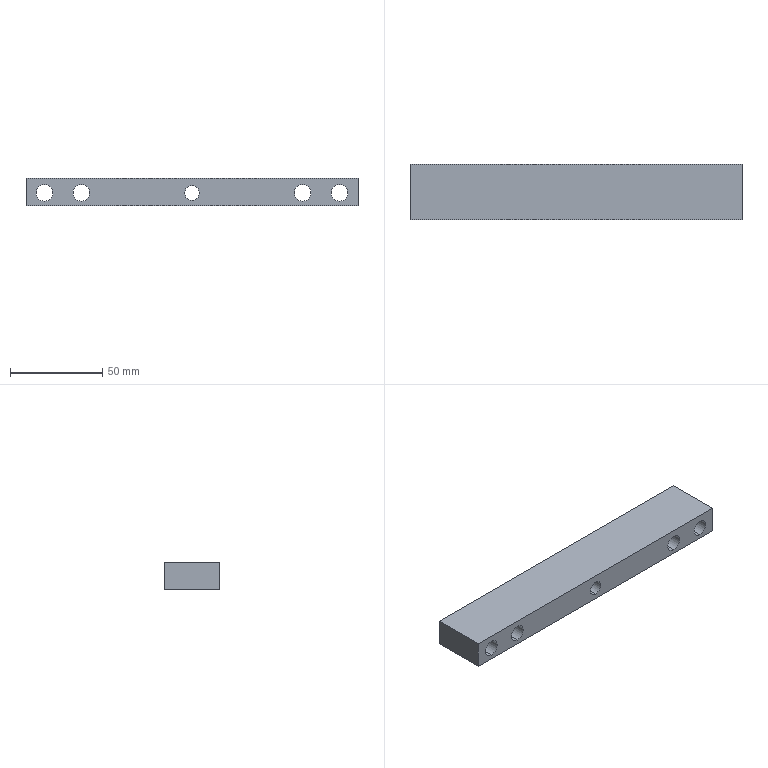Part | STEP file | J454-EBZ05-05-00-Part-1 | 1 solid | 16 faces | box 180 x 30 x 15 mm | volume 71858 mm3 | cylinder 10 | plane 6 | commonest cylinder face diameters 9 x8 8 x2
STEP:
#1=CARTESIAN_POINT('',(0.,0.,0.));
#2=DIRECTION('',(0.,0.,1.));
#3=DIRECTION('',(1.,0.,0.));
#4=AXIS2_PLACEMENT_3D('',#1,#2,#3);
#5=CARTESIAN_POINT('',(90.,0.,3.));
#6=VERTEX_POINT('',#5);
#7=CARTESIAN_POINT('',(90.,30.,3.));
#8=VERTEX_POINT('',#7);
#9=CARTESIAN_POINT('',(90.,0.,3.));
#10=DIRECTION('',(0.,1.,0.));
#11=VECTOR('',#10,1.);
#12=LINE('',#9,#11);
#13=CARTESIAN_POINT('',(90.,0.,7.));
#14=DIRECTION('',(0.,1.,0.));
#15=DIRECTION('',(0.,0.,-1.));
#16=AXIS2_PLACEMENT_3D('',#13,#14,#15);
#17=CYLINDRICAL_SURFACE('',#16,4.);
#18=CARTESIAN_POINT('',(6.283,0.));
#19=DIRECTION('',(0.,1.));
#20=VECTOR('',#19,1.);
#21=LINE('',#18,#20);
#22=(GEOMETRIC_REPRESENTATION_CONTEXT(2)PARAMETRIC_REPRESENTATION_CONTEXT()REPRESENTATION_CONTEXT('',''));
#23=DEFINITIONAL_REPRESENTATION('',(#21),#22);
#24=PCURVE('',#17,#23);
#25=CARTESIAN_POINT('',(90.,0.,7.));
#26=DIRECTION('',(0.,1.,0.));
#27=DIRECTION('',(0.,0.,-1.));
#28=AXIS2_PLACEMENT_3D('',#25,#26,#27);
#29=CYLINDRICAL_SURFACE('',#28,4.);
#30=CARTESIAN_POINT('',(0.,0.));
#31=DIRECTION('',(0.,1.));
#32=VECTOR('',#31,1.);
#33=LINE('',#30,#32);
#34=(GEOMETRIC_REPRESENTATION_CONTEXT(2)PARAMETRIC_REPRESENTATION_CONTEXT()REPRESENTATION_CONTEXT('',''));
#35=DEFINITIONAL_REPRESENTATION('',(#33),#34);
#36=PCURVE('',#29,#35);
#37=SURFACE_CURVE('',#12,(#24,#36),.PCURVE_S1.);
#38=EDGE_CURVE('',#6,#8,#37,.T.);
#39=ORIENTED_EDGE('',*,*,#38,.T.);
#40=CARTESIAN_POINT('',(90.,30.,11.));
#41=VERTEX_POINT('',#40);
#42=CARTESIAN_POINT('',(90.,30.,7.));
#43=DIRECTION('',(0.,-1.,0.));
#44=DIRECTION('',(0.,0.,1.));
#45=AXIS2_PLACEMENT_3D('',#42,#43,#44);
#46=CIRCLE('',#45,4.);
#47=CARTESIAN_POINT('',(9.425,30.));
#48=DIRECTION('',(-1.,0.));
#49=VECTOR('',#48,1.);
#50=LINE('',#47,#49);
#51=(GEOMETRIC_REPRESENTATION_CONTEXT(2)PARAMETRIC_REPRESENTATION_CONTEXT()REPRESENTATION_CONTEXT('',''));
#52=DEFINITIONAL_REPRESENTATION('',(#50),#51);
#53=PCURVE('',#17,#52);
#54=CARTESIAN_POINT('',(90.,30.,7.5));
#55=DIRECTION('',(0.,1.,0.));
#56=DIRECTION('',(0.,0.,-1.));
#57=AXIS2_PLACEMENT_3D('',#54,#55,#56);
#58=PLANE('',#57);
#59=CARTESIAN_POINT('',(-3.5,0.));
#60=CARTESIAN_POINT('',(-3.5,6.928));
#61=CARTESIAN_POINT('',(2.5,3.464));
#62=CARTESIAN_POINT('',(8.5,0.));
#63=CARTESIAN_POINT('',(2.5,-3.464));
#64=CARTESIAN_POINT('',(-3.5,-6.928));
#65=CARTESIAN_POINT('',(-3.5,0.));
#66=(BOUNDED_CURVE()B_SPLINE_CURVE(2,(#59,#60,#61,#62,#63,#64,#65),.UNSPECIFIED.,.T.,.F.)B_SPLINE_CURVE_WITH_KNOTS((1,2,2,2,2,1),(-2.094,0.,2.094,4.189,6.283,8.378),.UNSPECIFIED.)CURVE()GEOMETRIC_REPRESENTATION_ITEM()RATIONAL_B_SPLINE_CURVE((1.,0.5,1.,0.5,1.,0.5,1.))REPRESENTATION_ITEM(''));
#67=(GEOMETRIC_REPRESENTATION_CONTEXT(2)PARAMETRIC_REPRESENTATION_CONTEXT()REPRESENTATION_CONTEXT('',''));
#68=DEFINITIONAL_REPRESENTATION('',(#66),#67);
#69=PCURVE('',#58,#68);
#70=SURFACE_CURVE('',#46,(#53,#69),.PCURVE_S1.);
#71=EDGE_CURVE('',#8,#41,#70,.T.);
#72=ORIENTED_EDGE('',*,*,#71,.T.);
#73=CARTESIAN_POINT('',(90.,0.,11.));
#74=VERTEX_POINT('',#73);
#75=CARTESIAN_POINT('',(90.,0.,11.));
#76=DIRECTION('',(0.,1.,0.));
#77=VECTOR('',#76,1.);
#78=LINE('',#75,#77);
#79=CARTESIAN_POINT('',(3.142,0.));
#80=DIRECTION('',(0.,1.));
#81=VECTOR('',#80,1.);
#82=LINE('',#79,#81);
#83=(GEOMETRIC_REPRESENTATION_CONTEXT(2)PARAMETRIC_REPRESENTATION_CONTEXT()REPRESENTATION_CONTEXT('',''));
#84=DEFINITIONAL_REPRESENTATION('',(#82),#83);
#85=PCURVE('',#17,#84);
#86=CARTESIAN_POINT('',(3.142,0.));
#87=DIRECTION('',(0.,1.));
#88=VECTOR('',#87,1.);
#89=LINE('',#86,#88);
#90=(GEOMETRIC_REPRESENTATION_CONTEXT(2)PARAMETRIC_REPRESENTATION_CONTEXT()REPRESENTATION_CONTEXT('',''));
#91=DEFINITIONAL_REPRESENTATION('',(#89),#90);
#92=PCURVE('',#29,#91);
#93=SURFACE_CURVE('',#78,(#85,#92),.PCURVE_S1.);
#94=EDGE_CURVE('',#74,#41,#93,.T.);
#95=ORIENTED_EDGE('',*,*,#94,.F.);
#96=CARTESIAN_POINT('',(90.,0.,7.));
#97=DIRECTION('',(0.,1.,0.));
#98=DIRECTION('',(0.,0.,-1.));
#99=AXIS2_PLACEMENT_3D('',#96,#97,#98);
#100=CIRCLE('',#99,4.);
#101=CARTESIAN_POINT('',(0.,0.));
#102=DIRECTION('',(1.,0.));
#103=VECTOR('',#102,1.);
#104=LINE('',#101,#103);
#105=(GEOMETRIC_REPRESENTATION_CONTEXT(2)PARAMETRIC_REPRESENTATION_CONTEXT()REPRESENTATION_CONTEXT('',''));
#106=DEFINITIONAL_REPRESENTATION('',(#104),#105);
#107=PCURVE('',#17,#106);
#108=CARTESIAN_POINT('',(90.,0.,7.5));
#109=DIRECTION('',(0.,-1.,0.));
#110=DIRECTION('',(0.,0.,1.));
#111=AXIS2_PLACEMENT_3D('',#108,#109,#110);
#112=PLANE('',#111);
#113=CARTESIAN_POINT('',(-4.5,0.));
#114=CARTESIAN_POINT('',(-4.5,6.928));
#115=CARTESIAN_POINT('',(1.5,3.464));
#116=CARTESIAN_POINT('',(7.5,0.));
#117=CARTESIAN_POINT('',(1.5,-3.464));
#118=CARTESIAN_POINT('',(-4.5,-6.928));
#119=CARTESIAN_POINT('',(-4.5,0.));
#120=(BOUNDED_CURVE()B_SPLINE_CURVE(2,(#113,#114,#115,#116,#117,#118,#119),.UNSPECIFIED.,.T.,.F.)B_SPLINE_CURVE_WITH_KNOTS((1,2,2,2,2,1),(-2.094,0.,2.094,4.189,6.283,8.378),.UNSPECIFIED.)CURVE()GEOMETRIC_REPRESENTATION_ITEM()RATIONAL_B_SPLINE_CURVE((1.,0.5,1.,0.5,1.,0.5,1.))REPRESENTATION_ITEM(''));
#121=(GEOMETRIC_REPRESENTATION_CONTEXT(2)PARAMETRIC_REPRESENTATION_CONTEXT()REPRESENTATION_CONTEXT('',''));
#122=DEFINITIONAL_REPRESENTATION('',(#120),#121);
#123=PCURVE('',#112,#122);
#124=SURFACE_CURVE('',#100,(#107,#123),.PCURVE_S1.);
#125=EDGE_CURVE('',#74,#6,#124,.T.);
#126=ORIENTED_EDGE('',*,*,#125,.T.);
#127=EDGE_LOOP('',(#39,#72,#95,#126));
#128=FACE_BOUND('',#127,.F.);
#129=ADVANCED_FACE('',(#128),#17,.F.);
#130=CARTESIAN_POINT('',(170.,0.,2.5));
#131=VERTEX_POINT('',#130);
#132=CARTESIAN_POINT('',(170.,30.,2.5));
#133=VERTEX_POINT('',#132);
#134=CARTESIAN_POINT('',(170.,0.,2.5));
#135=DIRECTION('',(0.,1.,0.));
#136=VECTOR('',#135,1.);
#137=LINE('',#134,#136);
#138=CARTESIAN_POINT('',(170.,0.,7.));
#139=DIRECTION('',(0.,1.,0.));
#140=DIRECTION('',(0.,0.,-1.));
#141=AXIS2_PLACEMENT_3D('',#138,#139,#140);
#142=CYLINDRICAL_SURFACE('',#141,4.5);
#143=CARTESIAN_POINT('',(6.283,0.));
#144=DIRECTION('',(0.,1.));
#145=VECTOR('',#144,1.);
#146=LINE('',#143,#145);
#147=(GEOMETRIC_REPRESENTATION_CONTEXT(2)PARAMETRIC_REPRESENTATION_CONTEXT()REPRESENTATION_CONTEXT('',''));
#148=DEFINITIONAL_REPRESENTATION('',(#146),#147);
#149=PCURVE('',#142,#148);
#150=CARTESIAN_POINT('',(170.,0.,7.));
#151=DIRECTION('',(0.,1.,0.));
#152=DIRECTION('',(0.,0.,-1.));
#153=AXIS2_PLACEMENT_3D('',#150,#151,#152);
#154=CYLINDRICAL_SURFACE('',#153,4.5);
#155=CARTESIAN_POINT('',(0.,0.));
#156=DIRECTION('',(0.,1.));
#157=VECTOR('',#156,1.);
#158=LINE('',#155,#157);
#159=(GEOMETRIC_REPRESENTATION_CONTEXT(2)PARAMETRIC_REPRESENTATION_CONTEXT()REPRESENTATION_CONTEXT('',''));
#160=DEFINITIONAL_REPRESENTATION('',(#158),#159);
#161=PCURVE('',#154,#160);
#162=SURFACE_CURVE('',#137,(#149,#161),.PCURVE_S1.);
#163=EDGE_CURVE('',#131,#133,#162,.T.);
#164=ORIENTED_EDGE('',*,*,#163,.T.);
#165=CARTESIAN_POINT('',(170.,30.,11.5));
#166=VERTEX_POINT('',#165);
#167=CARTESIAN_POINT('',(170.,30.,7.));
#168=DIRECTION('',(0.,-1.,0.));
#169=DIRECTION('',(0.,0.,1.));
#170=AXIS2_PLACEMENT_3D('',#167,#168,#169);
#171=CIRCLE('',#170,4.5);
#172=CARTESIAN_POINT('',(9.425,30.));
#173=DIRECTION('',(-1.,0.));
#174=VECTOR('',#173,1.);
#175=LINE('',#172,#174);
#176=(GEOMETRIC_REPRESENTATION_CONTEXT(2)PARAMETRIC_REPRESENTATION_CONTEXT()REPRESENTATION_CONTEXT('',''));
#177=DEFINITIONAL_REPRESENTATION('',(#175),#176);
#178=PCURVE('',#142,#177);
#179=CARTESIAN_POINT('',(-4.,-80.));
#180=CARTESIAN_POINT('',(-4.,-72.206));
#181=CARTESIAN_POINT('',(2.75,-76.103));
#182=CARTESIAN_POINT('',(9.5,-80.));
#183=CARTESIAN_POINT('',(2.75,-83.897));
#184=CARTESIAN_POINT('',(-4.,-87.794));
#185=CARTESIAN_POINT('',(-4.,-80.));
#186=(BOUNDED_CURVE()B_SPLINE_CURVE(2,(#179,#180,#181,#182,#183,#184,#185),.UNSPECIFIED.,.T.,.F.)B_SPLINE_CURVE_WITH_KNOTS((1,2,2,2,2,1),(-2.094,0.,2.094,4.189,6.283,8.378),.UNSPECIFIED.)CURVE()GEOMETRIC_REPRESENTATION_ITEM()RATIONAL_B_SPLINE_CURVE((1.,0.5,1.,0.5,1.,0.5,1.))REPRESENTATION_ITEM(''));
#187=(GEOMETRIC_REPRESENTATION_CONTEXT(2)PARAMETRIC_REPRESENTATION_CONTEXT()REPRESENTATION_CONTEXT('',''));
#188=DEFINITIONAL_REPRESENTATION('',(#186),#187);
#189=PCURVE('',#58,#188);
#190=SURFACE_CURVE('',#171,(#178,#189),.PCURVE_S1.);
#191=EDGE_CURVE('',#133,#166,#190,.T.);
#192=ORIENTED_EDGE('',*,*,#191,.T.);
#193=CARTESIAN_POINT('',(170.,0.,11.5));
#194=VERTEX_POINT('',#193);
#195=CARTESIAN_POINT('',(170.,0.,11.5));
#196=DIRECTION('',(0.,1.,0.));
#197=VECTOR('',#196,1.);
#198=LINE('',#195,#197);
#199=CARTESIAN_POINT('',(3.142,0.));
#200=DIRECTION('',(0.,1.));
#201=VECTOR('',#200,1.);
#202=LINE('',#199,#201);
#203=(GEOMETRIC_REPRESENTATION_CONTEXT(2)PARAMETRIC_REPRESENTATION_CONTEXT()REPRESENTATION_CONTEXT('',''));
#204=DEFINITIONAL_REPRESENTATION('',(#202),#203);
#205=PCURVE('',#142,#204);
#206=CARTESIAN_POINT('',(3.142,0.));
#207=DIRECTION('',(0.,1.));
#208=VECTOR('',#207,1.);
#209=LINE('',#206,#208);
#210=(GEOMETRIC_REPRESENTATION_CONTEXT(2)PARAMETRIC_REPRESENTATION_CONTEXT()REPRESENTATION_CONTEXT('',''));
#211=DEFINITIONAL_REPRESENTATION('',(#209),#210);
#212=PCURVE('',#154,#211);
#213=SURFACE_CURVE('',#198,(#205,#212),.PCURVE_S1.);
#214=EDGE_CURVE('',#194,#166,#213,.T.);
#215=ORIENTED_EDGE('',*,*,#214,.F.);
#216=CARTESIAN_POINT('',(170.,0.,7.));
#217=DIRECTION('',(0.,1.,0.));
#218=DIRECTION('',(0.,0.,-1.));
#219=AXIS2_PLACEMENT_3D('',#216,#217,#218);
#220=CIRCLE('',#219,4.5);
#221=CARTESIAN_POINT('',(0.,0.));
#222=DIRECTION('',(1.,0.));
#223=VECTOR('',#222,1.);
#224=LINE('',#221,#223);
#225=(GEOMETRIC_REPRESENTATION_CONTEXT(2)PARAMETRIC_REPRESENTATION_CONTEXT()REPRESENTATION_CONTEXT('',''));
#226=DEFINITIONAL_REPRESENTATION('',(#224),#225);
#227=PCURVE('',#142,#226);
#228=CARTESIAN_POINT('',(-5.,-80.));
#229=CARTESIAN_POINT('',(-5.,-72.206));
#230=CARTESIAN_POINT('',(1.75,-76.103));
#231=CARTESIAN_POINT('',(8.5,-80.));
#232=CARTESIAN_POINT('',(1.75,-83.897));
#233=CARTESIAN_POINT('',(-5.,-87.794));
#234=CARTESIAN_POINT('',(-5.,-80.));
#235=(BOUNDED_CURVE()B_SPLINE_CURVE(2,(#228,#229,#230,#231,#232,#233,#234),.UNSPECIFIED.,.T.,.F.)B_SPLINE_CURVE_WITH_KNOTS((1,2,2,2,2,1),(-2.094,0.,2.094,4.189,6.283,8.378),.UNSPECIFIED.)CURVE()GEOMETRIC_REPRESENTATION_ITEM()RATIONAL_B_SPLINE_CURVE((1.,0.5,1.,0.5,1.,0.5,1.))REPRESENTATION_ITEM(''));
#236=(GEOMETRIC_REPRESENTATION_CONTEXT(2)PARAMETRIC_REPRESENTATION_CONTEXT()REPRESENTATION_CONTEXT('',''));
#237=DEFINITIONAL_REPRESENTATION('',(#235),#236);
#238=PCURVE('',#112,#237);
#239=SURFACE_CURVE('',#220,(#227,#238),.PCURVE_S1.);
#240=EDGE_CURVE('',#194,#131,#239,.T.);
#241=ORIENTED_EDGE('',*,*,#240,.T.);
#242=EDGE_LOOP('',(#164,#192,#215,#241));
#243=FACE_BOUND('',#242,.F.);
#244=ADVANCED_FACE('',(#243),#142,.F.);
#245=CARTESIAN_POINT('',(150.,0.,2.5));
#246=VERTEX_POINT('',#245);
#247=CARTESIAN_POINT('',(150.,30.,2.5));
#248=VERTEX_POINT('',#247);
#249=CARTESIAN_POINT('',(150.,0.,2.5));
#250=DIRECTION('',(0.,1.,0.));
#251=VECTOR('',#250,1.);
#252=LINE('',#249,#251);
#253=CARTESIAN_POINT('',(150.,0.,7.));
#254=DIRECTION('',(0.,1.,0.));
#255=DIRECTION('',(0.,0.,-1.));
#256=AXIS2_PLACEMENT_3D('',#253,#254,#255);
#257=CYLINDRICAL_SURFACE('',#256,4.5);
#258=CARTESIAN_POINT('',(6.283,0.));
#259=DIRECTION('',(0.,1.));
#260=VECTOR('',#259,1.);
#261=LINE('',#258,#260);
#262=(GEOMETRIC_REPRESENTATION_CONTEXT(2)PARAMETRIC_REPRESENTATION_CONTEXT()REPRESENTATION_CONTEXT('',''));
#263=DEFINITIONAL_REPRESENTATION('',(#261),#262);
#264=PCURVE('',#257,#263);
#265=CARTESIAN_POINT('',(150.,0.,7.));
#266=DIRECTION('',(0.,1.,0.));
#267=DIRECTION('',(0.,0.,-1.));
#268=AXIS2_PLACEMENT_3D('',#265,#266,#267);
#269=CYLINDRICAL_SURFACE('',#268,4.5);
#270=CARTESIAN_POINT('',(0.,0.));
#271=DIRECTION('',(0.,1.));
#272=VECTOR('',#271,1.);
#273=LINE('',#270,#272);
#274=(GEOMETRIC_REPRESENTATION_CONTEXT(2)PARAMETRIC_REPRESENTATION_CONTEXT()REPRESENTATION_CONTEXT('',''));
#275=DEFINITIONAL_REPRESENTATION('',(#273),#274);
#276=PCURVE('',#269,#275);
#277=SURFACE_CURVE('',#252,(#264,#276),.PCURVE_S1.);
#278=EDGE_CURVE('',#246,#248,#277,.T.);
#279=ORIENTED_EDGE('',*,*,#278,.T.);
#280=CARTESIAN_POINT('',(150.,30.,11.5));
#281=VERTEX_POINT('',#280);
#282=CARTESIAN_POINT('',(150.,30.,7.));
#283=DIRECTION('',(0.,-1.,0.));
#284=DIRECTION('',(0.,0.,1.));
#285=AXIS2_PLACEMENT_3D('',#282,#283,#284);
#286=CIRCLE('',#285,4.5);
#287=CARTESIAN_POINT('',(9.425,30.));
#288=DIRECTION('',(-1.,0.));
#289=VECTOR('',#288,1.);
#290=LINE('',#287,#289);
#291=(GEOMETRIC_REPRESENTATION_CONTEXT(2)PARAMETRIC_REPRESENTATION_CONTEXT()REPRESENTATION_CONTEXT('',''));
#292=DEFINITIONAL_REPRESENTATION('',(#290),#291);
#293=PCURVE('',#257,#292);
#294=CARTESIAN_POINT('',(-4.,-60.));
#295=CARTESIAN_POINT('',(-4.,-52.206));
#296=CARTESIAN_POINT('',(2.75,-56.103));
#297=CARTESIAN_POINT('',(9.5,-60.));
#298=CARTESIAN_POINT('',(2.75,-63.897));
#299=CARTESIAN_POINT('',(-4.,-67.794));
#300=CARTESIAN_POINT('',(-4.,-60.));
#301=(BOUNDED_CURVE()B_SPLINE_CURVE(2,(#294,#295,#296,#297,#298,#299,#300),.UNSPECIFIED.,.T.,.F.)B_SPLINE_CURVE_WITH_KNOTS((1,2,2,2,2,1),(-2.094,0.,2.094,4.189,6.283,8.378),.UNSPECIFIED.)CURVE()GEOMETRIC_REPRESENTATION_ITEM()RATIONAL_B_SPLINE_CURVE((1.,0.5,1.,0.5,1.,0.5,1.))REPRESENTATION_ITEM(''));
#302=(GEOMETRIC_REPRESENTATION_CONTEXT(2)PARAMETRIC_REPRESENTATION_CONTEXT()REPRESENTATION_CONTEXT('',''));
#303=DEFINITIONAL_REPRESENTATION('',(#301),#302);
#304=PCURVE('',#58,#303);
#305=SURFACE_CURVE('',#286,(#293,#304),.PCURVE_S1.);
#306=EDGE_CURVE('',#248,#281,#305,.T.);
#307=ORIENTED_EDGE('',*,*,#306,.T.);
#308=CARTESIAN_POINT('',(150.,0.,11.5));
#309=VERTEX_POINT('',#308);
#310=CARTESIAN_POINT('',(150.,0.,11.5));
#311=DIRECTION('',(0.,1.,0.));
#312=VECTOR('',#311,1.);
#313=LINE('',#310,#312);
#314=CARTESIAN_POINT('',(3.142,0.));
#315=DIRECTION('',(0.,1.));
#316=VECTOR('',#315,1.);
#317=LINE('',#314,#316);
#318=(GEOMETRIC_REPRESENTATION_CONTEXT(2)PARAMETRIC_REPRESENTATION_CONTEXT()REPRESENTATION_CONTEXT('',''));
#319=DEFINITIONAL_REPRESENTATION('',(#317),#318);
#320=PCURVE('',#257,#319);
#321=CARTESIAN_POINT('',(3.142,0.));
#322=DIRECTION('',(0.,1.));
#323=VECTOR('',#322,1.);
#324=LINE('',#321,#323);
#325=(GEOMETRIC_REPRESENTATION_CONTEXT(2)PARAMETRIC_REPRESENTATION_CONTEXT()REPRESENTATION_CONTEXT('',''));
#326=DEFINITIONAL_REPRESENTATION('',(#324),#325);
#327=PCURVE('',#269,#326);
#328=SURFACE_CURVE('',#313,(#320,#327),.PCURVE_S1.);
#329=EDGE_CURVE('',#309,#281,#328,.T.);
#330=ORIENTED_EDGE('',*,*,#329,.F.);
#331=CARTESIAN_POINT('',(150.,0.,7.));
#332=DIRECTION('',(0.,1.,0.));
#333=DIRECTION('',(0.,0.,-1.));
#334=AXIS2_PLACEMENT_3D('',#331,#332,#333);
#335=CIRCLE('',#334,4.5);
#336=CARTESIAN_POINT('',(0.,0.));
#337=DIRECTION('',(1.,0.));
#338=VECTOR('',#337,1.);
#339=LINE('',#336,#338);
#340=(GEOMETRIC_REPRESENTATION_CONTEXT(2)PARAMETRIC_REPRESENTATION_CONTEXT()REPRESENTATION_CONTEXT('',''));
#341=DEFINITIONAL_REPRESENTATION('',(#339),#340);
#342=PCURVE('',#257,#341);
#343=CARTESIAN_POINT('',(-5.,-60.));
#344=CARTESIAN_POINT('',(-5.,-52.206));
#345=CARTESIAN_POINT('',(1.75,-56.103));
#346=CARTESIAN_POINT('',(8.5,-60.));
#347=CARTESIAN_POINT('',(1.75,-63.897));
#348=CARTESIAN_POINT('',(-5.,-67.794));
#349=CARTESIAN_POINT('',(-5.,-60.));
#350=(BOUNDED_CURVE()B_SPLINE_CURVE(2,(#343,#344,#345,#346,#347,#348,#349),.UNSPECIFIED.,.T.,.F.)B_SPLINE_CURVE_WITH_KNOTS((1,2,2,2,2,1),(-2.094,0.,2.094,4.189,6.283,8.378),.UNSPECIFIED.)CURVE()GEOMETRIC_REPRESENTATION_ITEM()RATIONAL_B_SPLINE_CURVE((1.,0.5,1.,0.5,1.,0.5,1.))REPRESENTATION_ITEM(''));
#351=(GEOMETRIC_REPRESENTATION_CONTEXT(2)PARAMETRIC_REPRESENTATION_CONTEXT()REPRESENTATION_CONTEXT('',''));
#352=DEFINITIONAL_REPRESENTATION('',(#350),#351);
#353=PCURVE('',#112,#352);
#354=SURFACE_CURVE('',#335,(#342,#353),.PCURVE_S1.);
#355=EDGE_CURVE('',#309,#246,#354,.T.);
#356=ORIENTED_EDGE('',*,*,#355,.T.);
#357=EDGE_LOOP('',(#279,#307,#330,#356));
#358=FACE_BOUND('',#357,.F.);
#359=ADVANCED_FACE('',(#358),#257,.F.);
#360=CARTESIAN_POINT('',(30.,0.,2.5));
#361=VERTEX_POINT('',#360);
#362=CARTESIAN_POINT('',(30.,30.,2.5));
#363=VERTEX_POINT('',#362);
#364=CARTESIAN_POINT('',(30.,0.,2.5));
#365=DIRECTION('',(0.,1.,0.));
#366=VECTOR('',#365,1.);
#367=LINE('',#364,#366);
#368=CARTESIAN_POINT('',(30.,0.,7.));
#369=DIRECTION('',(0.,1.,0.));
#370=DIRECTION('',(0.,0.,-1.));
#371=AXIS2_PLACEMENT_3D('',#368,#369,#370);
#372=CYLINDRICAL_SURFACE('',#371,4.5);
#373=CARTESIAN_POINT('',(6.283,0.));
#374=DIRECTION('',(0.,1.));
#375=VECTOR('',#374,1.);
#376=LINE('',#373,#375);
#377=(GEOMETRIC_REPRESENTATION_CONTEXT(2)PARAMETRIC_REPRESENTATION_CONTEXT()REPRESENTATION_CONTEXT('',''));
#378=DEFINITIONAL_REPRESENTATION('',(#376),#377);
#379=PCURVE('',#372,#378);
#380=CARTESIAN_POINT('',(30.,0.,7.));
#381=DIRECTION('',(0.,1.,0.));
#382=DIRECTION('',(0.,0.,-1.));
#383=AXIS2_PLACEMENT_3D('',#380,#381,#382);
#384=CYLINDRICAL_SURFACE('',#383,4.5);
#385=CARTESIAN_POINT('',(0.,0.));
#386=DIRECTION('',(0.,1.));
#387=VECTOR('',#386,1.);
#388=LINE('',#385,#387);
#389=(GEOMETRIC_REPRESENTATION_CONTEXT(2)PARAMETRIC_REPRESENTATION_CONTEXT()REPRESENTATION_CONTEXT('',''));
#390=DEFINITIONAL_REPRESENTATION('',(#388),#389);
#391=PCURVE('',#384,#390);
#392=SURFACE_CURVE('',#367,(#379,#391),.PCURVE_S1.);
#393=EDGE_CURVE('',#361,#363,#392,.T.);
#394=ORIENTED_EDGE('',*,*,#393,.T.);
#395=CARTESIAN_POINT('',(30.,30.,11.5));
#396=VERTEX_POINT('',#395);
#397=CARTESIAN_POINT('',(30.,30.,7.));
#398=DIRECTION('',(0.,-1.,0.));
#399=DIRECTION('',(0.,0.,1.));
#400=AXIS2_PLACEMENT_3D('',#397,#398,#399);
#401=CIRCLE('',#400,4.5);
#402=CARTESIAN_POINT('',(9.425,30.));
#403=DIRECTION('',(-1.,0.));
#404=VECTOR('',#403,1.);
#405=LINE('',#402,#404);
#406=(GEOMETRIC_REPRESENTATION_CONTEXT(2)PARAMETRIC_REPRESENTATION_CONTEXT()REPRESENTATION_CONTEXT('',''));
#407=DEFINITIONAL_REPRESENTATION('',(#405),#406);
#408=PCURVE('',#372,#407);
#409=CARTESIAN_POINT('',(-4.,60.));
#410=CARTESIAN_POINT('',(-4.,67.794));
#411=CARTESIAN_POINT('',(2.75,63.897));
#412=CARTESIAN_POINT('',(9.5,60.));
#413=CARTESIAN_POINT('',(2.75,56.103));
#414=CARTESIAN_POINT('',(-4.,52.206));
#415=CARTESIAN_POINT('',(-4.,60.));
#416=(BOUNDED_CURVE()B_SPLINE_CURVE(2,(#409,#410,#411,#412,#413,#414,#415),.UNSPECIFIED.,.T.,.F.)B_SPLINE_CURVE_WITH_KNOTS((1,2,2,2,2,1),(-2.094,0.,2.094,4.189,6.283,8.378),.UNSPECIFIED.)CURVE()GEOMETRIC_REPRESENTATION_ITEM()RATIONAL_B_SPLINE_CURVE((1.,0.5,1.,0.5,1.,0.5,1.))REPRESENTATION_ITEM(''));
#417=(GEOMETRIC_REPRESENTATION_CONTEXT(2)PARAMETRIC_REPRESENTATION_CONTEXT()REPRESENTATION_CONTEXT('',''));
#418=DEFINITIONAL_REPRESENTATION('',(#416),#417);
#419=PCURVE('',#58,#418);
#420=SURFACE_CURVE('',#401,(#408,#419),.PCURVE_S1.);
#421=EDGE_CURVE('',#363,#396,#420,.T.);
#422=ORIENTED_EDGE('',*,*,#421,.T.);
#423=CARTESIAN_POINT('',(30.,0.,11.5));
#424=VERTEX_POINT('',#423);
#425=CARTESIAN_POINT('',(30.,0.,11.5));
#426=DIRECTION('',(0.,1.,0.));
#427=VECTOR('',#426,1.);
#428=LINE('',#425,#427);
#429=CARTESIAN_POINT('',(3.142,0.));
#430=DIRECTION('',(0.,1.));
#431=VECTOR('',#430,1.);
#432=LINE('',#429,#431);
#433=(GEOMETRIC_REPRESENTATION_CONTEXT(2)PARAMETRIC_REPRESENTATION_CONTEXT()REPRESENTATION_CONTEXT('',''));
#434=DEFINITIONAL_REPRESENTATION('',(#432),#433);
#435=PCURVE('',#372,#434);
#436=CARTESIAN_POINT('',(3.142,0.));
#437=DIRECTION('',(0.,1.));
#438=VECTOR('',#437,1.);
#439=LINE('',#436,#438);
#440=(GEOMETRIC_REPRESENTATION_CONTEXT(2)PARAMETRIC_REPRESENTATION_CONTEXT()REPRESENTATION_CONTEXT('',''));
#441=DEFINITIONAL_REPRESENTATION('',(#439),#440);
#442=PCURVE('',#384,#441);
#443=SURFACE_CURVE('',#428,(#435,#442),.PCURVE_S1.);
#444=EDGE_CURVE('',#424,#396,#443,.T.);
#445=ORIENTED_EDGE('',*,*,#444,.F.);
#446=CARTESIAN_POINT('',(30.,0.,7.));
#447=DIRECTION('',(0.,1.,0.));
#448=DIRECTION('',(0.,0.,-1.));
#449=AXIS2_PLACEMENT_3D('',#446,#447,#448);
#450=CIRCLE('',#449,4.5);
#451=CARTESIAN_POINT('',(0.,0.));
#452=DIRECTION('',(1.,0.));
#453=VECTOR('',#452,1.);
#454=LINE('',#451,#453);
#455=(GEOMETRIC_REPRESENTATION_CONTEXT(2)PARAMETRIC_REPRESENTATION_CONTEXT()REPRESENTATION_CONTEXT('',''));
#456=DEFINITIONAL_REPRESENTATION('',(#454),#455);
#457=PCURVE('',#372,#456);
#458=CARTESIAN_POINT('',(-5.,60.));
#459=CARTESIAN_POINT('',(-5.,67.794));
#460=CARTESIAN_POINT('',(1.75,63.897));
#461=CARTESIAN_POINT('',(8.5,60.));
#462=CARTESIAN_POINT('',(1.75,56.103));
#463=CARTESIAN_POINT('',(-5.,52.206));
#464=CARTESIAN_POINT('',(-5.,60.));
#465=(BOUNDED_CURVE()B_SPLINE_CURVE(2,(#458,#459,#460,#461,#462,#463,#464),.UNSPECIFIED.,.T.,.F.)B_SPLINE_CURVE_WITH_KNOTS((1,2,2,2,2,1),(-2.094,0.,2.094,4.189,6.283,8.378),.UNSPECIFIED.)CURVE()GEOMETRIC_REPRESENTATION_ITEM()RATIONAL_B_SPLINE_CURVE((1.,0.5,1.,0.5,1.,0.5,1.))REPRESENTATION_ITEM(''));
#466=(GEOMETRIC_REPRESENTATION_CONTEXT(2)PARAMETRIC_REPRESENTATION_CONTEXT()REPRESENTATION_CONTEXT('',''));
#467=DEFINITIONAL_REPRESENTATION('',(#465),#466);
#468=PCURVE('',#112,#467);
#469=SURFACE_CURVE('',#450,(#457,#468),.PCURVE_S1.);
#470=EDGE_CURVE('',#424,#361,#469,.T.);
#471=ORIENTED_EDGE('',*,*,#470,.T.);
#472=EDGE_LOOP('',(#394,#422,#445,#471));
#473=FACE_BOUND('',#472,.F.);
#474=ADVANCED_FACE('',(#473),#372,.F.);
#475=CARTESIAN_POINT('',(10.,0.,2.5));
#476=VERTEX_POINT('',#475);
#477=CARTESIAN_POINT('',(10.,30.,2.5));
#478=VERTEX_POINT('',#477);
#479=CARTESIAN_POINT('',(10.,0.,2.5));
#480=DIRECTION('',(0.,1.,0.));
#481=VECTOR('',#480,1.);
#482=LINE('',#479,#481);
#483=CARTESIAN_POINT('',(10.,0.,7.));
#484=DIRECTION('',(0.,1.,0.));
#485=DIRECTION('',(0.,0.,-1.));
#486=AXIS2_PLACEMENT_3D('',#483,#484,#485);
#487=CYLINDRICAL_SURFACE('',#486,4.5);
#488=CARTESIAN_POINT('',(6.283,0.));
#489=DIRECTION('',(0.,1.));
#490=VECTOR('',#489,1.);
#491=LINE('',#488,#490);
#492=(GEOMETRIC_REPRESENTATION_CONTEXT(2)PARAMETRIC_REPRESENTATION_CONTEXT()REPRESENTATION_CONTEXT('',''));
#493=DEFINITIONAL_REPRESENTATION('',(#491),#492);
#494=PCURVE('',#487,#493);
#495=CARTESIAN_POINT('',(10.,0.,7.));
#496=DIRECTION('',(0.,1.,0.));
#497=DIRECTION('',(0.,0.,-1.));
#498=AXIS2_PLACEMENT_3D('',#495,#496,#497);
#499=CYLINDRICAL_SURFACE('',#498,4.5);
#500=CARTESIAN_POINT('',(0.,0.));
#501=DIRECTION('',(0.,1.));
#502=VECTOR('',#501,1.);
#503=LINE('',#500,#502);
#504=(GEOMETRIC_REPRESENTATION_CONTEXT(2)PARAMETRIC_REPRESENTATION_CONTEXT()REPRESENTATION_CONTEXT('',''));
#505=DEFINITIONAL_REPRESENTATION('',(#503),#504);
#506=PCURVE('',#499,#505);
#507=SURFACE_CURVE('',#482,(#494,#506),.PCURVE_S1.);
#508=EDGE_CURVE('',#476,#478,#507,.T.);
#509=ORIENTED_EDGE('',*,*,#508,.T.);
#510=CARTESIAN_POINT('',(10.,30.,11.5));
#511=VERTEX_POINT('',#510);
#512=CARTESIAN_POINT('',(10.,30.,7.));
#513=DIRECTION('',(0.,-1.,0.));
#514=DIRECTION('',(0.,0.,1.));
#515=AXIS2_PLACEMENT_3D('',#512,#513,#514);
#516=CIRCLE('',#515,4.5);
#517=CARTESIAN_POINT('',(9.425,30.));
#518=DIRECTION('',(-1.,0.));
#519=VECTOR('',#518,1.);
#520=LINE('',#517,#519);
#521=(GEOMETRIC_REPRESENTATION_CONTEXT(2)PARAMETRIC_REPRESENTATION_CONTEXT()REPRESENTATION_CONTEXT('',''));
#522=DEFINITIONAL_REPRESENTATION('',(#520),#521);
#523=PCURVE('',#487,#522);
#524=CARTESIAN_POINT('',(-4.,80.));
#525=CARTESIAN_POINT('',(-4.,87.794));
#526=CARTESIAN_POINT('',(2.75,83.897));
#527=CARTESIAN_POINT('',(9.5,80.));
#528=CARTESIAN_POINT('',(2.75,76.103));
#529=CARTESIAN_POINT('',(-4.,72.206));
#530=CARTESIAN_POINT('',(-4.,80.));
#531=(BOUNDED_CURVE()B_SPLINE_CURVE(2,(#524,#525,#526,#527,#528,#529,#530),.UNSPECIFIED.,.T.,.F.)B_SPLINE_CURVE_WITH_KNOTS((1,2,2,2,2,1),(-2.094,0.,2.094,4.189,6.283,8.378),.UNSPECIFIED.)CURVE()GEOMETRIC_REPRESENTATION_ITEM()RATIONAL_B_SPLINE_CURVE((1.,0.5,1.,0.5,1.,0.5,1.))REPRESENTATION_ITEM(''));
#532=(GEOMETRIC_REPRESENTATION_CONTEXT(2)PARAMETRIC_REPRESENTATION_CONTEXT()REPRESENTATION_CONTEXT('',''));
#533=DEFINITIONAL_REPRESENTATION('',(#531),#532);
#534=PCURVE('',#58,#533);
#535=SURFACE_CURVE('',#516,(#523,#534),.PCURVE_S1.);
#536=EDGE_CURVE('',#478,#511,#535,.T.);
#537=ORIENTED_EDGE('',*,*,#536,.T.);
#538=CARTESIAN_POINT('',(10.,0.,11.5));
#539=VERTEX_POINT('',#538);
#540=CARTESIAN_POINT('',(10.,0.,11.5));
#541=DIRECTION('',(0.,1.,0.));
#542=VECTOR('',#541,1.);
#543=LINE('',#540,#542);
#544=CARTESIAN_POINT('',(3.142,0.));
#545=DIRECTION('',(0.,1.));
#546=VECTOR('',#545,1.);
#547=LINE('',#544,#546);
#548=(GEOMETRIC_REPRESENTATION_CONTEXT(2)PARAMETRIC_REPRESENTATION_CONTEXT()REPRESENTATION_CONTEXT('',''));
#549=DEFINITIONAL_REPRESENTATION('',(#547),#548);
#550=PCURVE('',#487,#549);
#551=CARTESIAN_POINT('',(3.142,0.));
#552=DIRECTION('',(0.,1.));
#553=VECTOR('',#552,1.);
#554=LINE('',#551,#553);
#555=(GEOMETRIC_REPRESENTATION_CONTEXT(2)PARAMETRIC_REPRESENTATION_CONTEXT()REPRESENTATION_CONTEXT('',''));
#556=DEFINITIONAL_REPRESENTATION('',(#554),#555);
#557=PCURVE('',#499,#556);
#558=SURFACE_CURVE('',#543,(#550,#557),.PCURVE_S1.);
#559=EDGE_CURVE('',#539,#511,#558,.T.);
#560=ORIENTED_EDGE('',*,*,#559,.F.);
#561=CARTESIAN_POINT('',(10.,0.,7.));
#562=DIRECTION('',(0.,1.,0.));
#563=DIRECTION('',(0.,0.,-1.));
#564=AXIS2_PLACEMENT_3D('',#561,#562,#563);
#565=CIRCLE('',#564,4.5);
#566=CARTESIAN_POINT('',(0.,0.));
#567=DIRECTION('',(1.,0.));
#568=VECTOR('',#567,1.);
#569=LINE('',#566,#568);
#570=(GEOMETRIC_REPRESENTATION_CONTEXT(2)PARAMETRIC_REPRESENTATION_CONTEXT()REPRESENTATION_CONTEXT('',''));
#571=DEFINITIONAL_REPRESENTATION('',(#569),#570);
#572=PCURVE('',#487,#571);
#573=CARTESIAN_POINT('',(-5.,80.));
#574=CARTESIAN_POINT('',(-5.,87.794));
#575=CARTESIAN_POINT('',(1.75,83.897));
#576=CARTESIAN_POINT('',(8.5,80.));
#577=CARTESIAN_POINT('',(1.75,76.103));
#578=CARTESIAN_POINT('',(-5.,72.206));
#579=CARTESIAN_POINT('',(-5.,80.));
#580=(BOUNDED_CURVE()B_SPLINE_CURVE(2,(#573,#574,#575,#576,#577,#578,#579),.UNSPECIFIED.,.T.,.F.)B_SPLINE_CURVE_WITH_KNOTS((1,2,2,2,2,1),(-2.094,0.,2.094,4.189,6.283,8.378),.UNSPECIFIED.)CURVE()GEOMETRIC_REPRESENTATION_ITEM()RATIONAL_B_SPLINE_CURVE((1.,0.5,1.,0.5,1.,0.5,1.))REPRESENTATION_ITEM(''));
#581=(GEOMETRIC_REPRESENTATION_CONTEXT(2)PARAMETRIC_REPRESENTATION_CONTEXT()REPRESENTATION_CONTEXT('',''));
#582=DEFINITIONAL_REPRESENTATION('',(#580),#581);
#583=PCURVE('',#112,#582);
#584=SURFACE_CURVE('',#565,(#572,#583),.PCURVE_S1.);
#585=EDGE_CURVE('',#539,#476,#584,.T.);
#586=ORIENTED_EDGE('',*,*,#585,.T.);
#587=EDGE_LOOP('',(#509,#537,#560,#586));
#588=FACE_BOUND('',#587,.F.);
#589=ADVANCED_FACE('',(#588),#487,.F.);
#590=CARTESIAN_POINT('',(90.,0.,7.));
#591=DIRECTION('',(0.,1.,0.));
#592=DIRECTION('',(0.,0.,-1.));
#593=AXIS2_PLACEMENT_3D('',#590,#591,#592);
#594=CIRCLE('',#593,4.);
#595=CARTESIAN_POINT('',(-4.5,0.));
#596=CARTESIAN_POINT('',(-4.5,6.928));
#597=CARTESIAN_POINT('',(1.5,3.464));
#598=CARTESIAN_POINT('',(7.5,0.));
#599=CARTESIAN_POINT('',(1.5,-3.464));
#600=CARTESIAN_POINT('',(-4.5,-6.928));
#601=CARTESIAN_POINT('',(-4.5,0.));
#602=(BOUNDED_CURVE()B_SPLINE_CURVE(2,(#595,#596,#597,#598,#599,#600,#601),.UNSPECIFIED.,.T.,.F.)B_SPLINE_CURVE_WITH_KNOTS((1,2,2,2,2,1),(-2.094,0.,2.094,4.189,6.283,8.378),.UNSPECIFIED.)CURVE()GEOMETRIC_REPRESENTATION_ITEM()RATIONAL_B_SPLINE_CURVE((1.,0.5,1.,0.5,1.,0.5,1.))REPRESENTATION_ITEM(''));
#603=(GEOMETRIC_REPRESENTATION_CONTEXT(2)PARAMETRIC_REPRESENTATION_CONTEXT()REPRESENTATION_CONTEXT('',''));
#604=DEFINITIONAL_REPRESENTATION('',(#602),#603);
#605=PCURVE('',#112,#604);
#606=CARTESIAN_POINT('',(0.,0.));
#607=DIRECTION('',(1.,0.));
#608=VECTOR('',#607,1.);
#609=LINE('',#606,#608);
#610=(GEOMETRIC_REPRESENTATION_CONTEXT(2)PARAMETRIC_REPRESENTATION_CONTEXT()REPRESENTATION_CONTEXT('',''));
#611=DEFINITIONAL_REPRESENTATION('',(#609),#610);
#612=PCURVE('',#29,#611);
#613=SURFACE_CURVE('',#594,(#605,#612),.PCURVE_S1.);
#614=EDGE_CURVE('',#6,#74,#613,.T.);
#615=ORIENTED_EDGE('',*,*,#614,.T.);
#616=ORIENTED_EDGE('',*,*,#125,.T.);
#617=EDGE_LOOP('',(#615,#616));
#618=FACE_BOUND('',#617,.T.);
#619=CARTESIAN_POINT('',(170.,0.,7.));
#620=DIRECTION('',(0.,1.,0.));
#621=DIRECTION('',(0.,0.,-1.));
#622=AXIS2_PLACEMENT_3D('',#619,#620,#621);
#623=CIRCLE('',#622,4.5);
#624=CARTESIAN_POINT('',(-5.,-80.));
#625=CARTESIAN_POINT('',(-5.,-72.206));
#626=CARTESIAN_POINT('',(1.75,-76.103));
#627=CARTESIAN_POINT('',(8.5,-80.));
#628=CARTESIAN_POINT('',(1.75,-83.897));
#629=CARTESIAN_POINT('',(-5.,-87.794));
#630=CARTESIAN_POINT('',(-5.,-80.));
#631=(BOUNDED_CURVE()B_SPLINE_CURVE(2,(#624,#625,#626,#627,#628,#629,#630),.UNSPECIFIED.,.T.,.F.)B_SPLINE_CURVE_WITH_KNOTS((1,2,2,2,2,1),(-2.094,0.,2.094,4.189,6.283,8.378),.UNSPECIFIED.)CURVE()GEOMETRIC_REPRESENTATION_ITEM()RATIONAL_B_SPLINE_CURVE((1.,0.5,1.,0.5,1.,0.5,1.))REPRESENTATION_ITEM(''));
#632=(GEOMETRIC_REPRESENTATION_CONTEXT(2)PARAMETRIC_REPRESENTATION_CONTEXT()REPRESENTATION_CONTEXT('',''));
#633=DEFINITIONAL_REPRESENTATION('',(#631),#632);
#634=PCURVE('',#112,#633);
#635=CARTESIAN_POINT('',(0.,0.));
#636=DIRECTION('',(1.,0.));
#637=VECTOR('',#636,1.);
#638=LINE('',#635,#637);
#639=(GEOMETRIC_REPRESENTATION_CONTEXT(2)PARAMETRIC_REPRESENTATION_CONTEXT()REPRESENTATION_CONTEXT('',''));
#640=DEFINITIONAL_REPRESENTATION('',(#638),#639);
#641=PCURVE('',#154,#640);
#642=SURFACE_CURVE('',#623,(#634,#641),.PCURVE_S1.);
#643=EDGE_CURVE('',#131,#194,#642,.T.);
#644=ORIENTED_EDGE('',*,*,#643,.T.);
#645=ORIENTED_EDGE('',*,*,#240,.T.);
#646=EDGE_LOOP('',(#644,#645));
#647=FACE_BOUND('',#646,.T.);
#648=CARTESIAN_POINT('',(150.,0.,7.));
#649=DIRECTION('',(0.,1.,0.));
#650=DIRECTION('',(0.,0.,-1.));
#651=AXIS2_PLACEMENT_3D('',#648,#649,#650);
#652=CIRCLE('',#651,4.5);
#653=CARTESIAN_POINT('',(-5.,-60.));
#654=CARTESIAN_POINT('',(-5.,-52.206));
#655=CARTESIAN_POINT('',(1.75,-56.103));
#656=CARTESIAN_POINT('',(8.5,-60.));
#657=CARTESIAN_POINT('',(1.75,-63.897));
#658=CARTESIAN_POINT('',(-5.,-67.794));
#659=CARTESIAN_POINT('',(-5.,-60.));
#660=(BOUNDED_CURVE()B_SPLINE_CURVE(2,(#653,#654,#655,#656,#657,#658,#659),.UNSPECIFIED.,.T.,.F.)B_SPLINE_CURVE_WITH_KNOTS((1,2,2,2,2,1),(-2.094,0.,2.094,4.189,6.283,8.378),.UNSPECIFIED.)CURVE()GEOMETRIC_REPRESENTATION_ITEM()RATIONAL_B_SPLINE_CURVE((1.,0.5,1.,0.5,1.,0.5,1.))REPRESENTATION_ITEM(''));
#661=(GEOMETRIC_REPRESENTATION_CONTEXT(2)PARAMETRIC_REPRESENTATION_CONTEXT()REPRESENTATION_CONTEXT('',''));
#662=DEFINITIONAL_REPRESENTATION('',(#660),#661);
#663=PCURVE('',#112,#662);
#664=CARTESIAN_POINT('',(0.,0.));
#665=DIRECTION('',(1.,0.));
#666=VECTOR('',#665,1.);
#667=LINE('',#664,#666);
#668=(GEOMETRIC_REPRESENTATION_CONTEXT(2)PARAMETRIC_REPRESENTATION_CONTEXT()REPRESENTATION_CONTEXT('',''));
#669=DEFINITIONAL_REPRESENTATION('',(#667),#668);
#670=PCURVE('',#269,#669);
#671=SURFACE_CURVE('',#652,(#663,#670),.PCURVE_S1.);
#672=EDGE_CURVE('',#246,#309,#671,.T.);
#673=ORIENTED_EDGE('',*,*,#672,.T.);
#674=ORIENTED_EDGE('',*,*,#355,.T.);
#675=EDGE_LOOP('',(#673,#674));
#676=FACE_BOUND('',#675,.T.);
#677=CARTESIAN_POINT('',(30.,0.,7.));
#678=DIRECTION('',(0.,1.,0.));
#679=DIRECTION('',(0.,0.,-1.));
#680=AXIS2_PLACEMENT_3D('',#677,#678,#679);
#681=CIRCLE('',#680,4.5);
#682=CARTESIAN_POINT('',(-5.,60.));
#683=CARTESIAN_POINT('',(-5.,67.794));
#684=CARTESIAN_POINT('',(1.75,63.897));
#685=CARTESIAN_POINT('',(8.5,60.));
#686=CARTESIAN_POINT('',(1.75,56.103));
#687=CARTESIAN_POINT('',(-5.,52.206));
#688=CARTESIAN_POINT('',(-5.,60.));
#689=(BOUNDED_CURVE()B_SPLINE_CURVE(2,(#682,#683,#684,#685,#686,#687,#688),.UNSPECIFIED.,.T.,.F.)B_SPLINE_CURVE_WITH_KNOTS((1,2,2,2,2,1),(-2.094,0.,2.094,4.189,6.283,8.378),.UNSPECIFIED.)CURVE()GEOMETRIC_REPRESENTATION_ITEM()RATIONAL_B_SPLINE_CURVE((1.,0.5,1.,0.5,1.,0.5,1.))REPRESENTATION_ITEM(''));
#690=(GEOMETRIC_REPRESENTATION_CONTEXT(2)PARAMETRIC_REPRESENTATION_CONTEXT()REPRESENTATION_CONTEXT('',''));
#691=DEFINITIONAL_REPRESENTATION('',(#689),#690);
#692=PCURVE('',#112,#691);
#693=CARTESIAN_POINT('',(0.,0.));
#694=DIRECTION('',(1.,0.));
#695=VECTOR('',#694,1.);
#696=LINE('',#693,#695);
#697=(GEOMETRIC_REPRESENTATION_CONTEXT(2)PARAMETRIC_REPRESENTATION_CONTEXT()REPRESENTATION_CONTEXT('',''));
#698=DEFINITIONAL_REPRESENTATION('',(#696),#697);
#699=PCURVE('',#384,#698);
#700=SURFACE_CURVE('',#681,(#692,#699),.PCURVE_S1.);
#701=EDGE_CURVE('',#361,#424,#700,.T.);
#702=ORIENTED_EDGE('',*,*,#701,.T.);
#703=ORIENTED_EDGE('',*,*,#470,.T.);
#704=EDGE_LOOP('',(#702,#703));
#705=FACE_BOUND('',#704,.T.);
#706=CARTESIAN_POINT('',(10.,0.,7.));
#707=DIRECTION('',(0.,1.,0.));
#708=DIRECTION('',(0.,0.,-1.));
#709=AXIS2_PLACEMENT_3D('',#706,#707,#708);
#710=CIRCLE('',#709,4.5);
#711=CARTESIAN_POINT('',(-5.,80.));
#712=CARTESIAN_POINT('',(-5.,87.794));
#713=CARTESIAN_POINT('',(1.75,83.897));
#714=CARTESIAN_POINT('',(8.5,80.));
#715=CARTESIAN_POINT('',(1.75,76.103));
#716=CARTESIAN_POINT('',(-5.,72.206));
#717=CARTESIAN_POINT('',(-5.,80.));
#718=(BOUNDED_CURVE()B_SPLINE_CURVE(2,(#711,#712,#713,#714,#715,#716,#717),.UNSPECIFIED.,.T.,.F.)B_SPLINE_CURVE_WITH_KNOTS((1,2,2,2,2,1),(-2.094,0.,2.094,4.189,6.283,8.378),.UNSPECIFIED.)CURVE()GEOMETRIC_REPRESENTATION_ITEM()RATIONAL_B_SPLINE_CURVE((1.,0.5,1.,0.5,1.,0.5,1.))REPRESENTATION_ITEM(''));
#719=(GEOMETRIC_REPRESENTATION_CONTEXT(2)PARAMETRIC_REPRESENTATION_CONTEXT()REPRESENTATION_CONTEXT('',''));
#720=DEFINITIONAL_REPRESENTATION('',(#718),#719);
#721=PCURVE('',#112,#720);
#722=CARTESIAN_POINT('',(0.,0.));
#723=DIRECTION('',(1.,0.));
#724=VECTOR('',#723,1.);
#725=LINE('',#722,#724);
#726=(GEOMETRIC_REPRESENTATION_CONTEXT(2)PARAMETRIC_REPRESENTATION_CONTEXT()REPRESENTATION_CONTEXT('',''));
#727=DEFINITIONAL_REPRESENTATION('',(#725),#726);
#728=PCURVE('',#499,#727);
#729=SURFACE_CURVE('',#710,(#721,#728),.PCURVE_S1.);
#730=EDGE_CURVE('',#476,#539,#729,.T.);
#731=ORIENTED_EDGE('',*,*,#730,.T.);
#732=ORIENTED_EDGE('',*,*,#585,.T.);
#733=EDGE_LOOP('',(#731,#732));
#734=FACE_BOUND('',#733,.T.);
#735=CARTESIAN_POINT('',(180.,0.,15.));
#736=VERTEX_POINT('',#735);
#737=CARTESIAN_POINT('',(180.,0.,0.));
#738=VERTEX_POINT('',#737);
#739=CARTESIAN_POINT('',(180.,0.,7.5));
#740=DIRECTION('',(0.,0.,-1.));
#741=VECTOR('',#740,1.);
#742=LINE('',#739,#741);
#743=CARTESIAN_POINT('',(0.,-90.));
#744=DIRECTION('',(-1.,0.));
#745=VECTOR('',#744,1.);
#746=LINE('',#743,#745);
#747=(GEOMETRIC_REPRESENTATION_CONTEXT(2)PARAMETRIC_REPRESENTATION_CONTEXT()REPRESENTATION_CONTEXT('',''));
#748=DEFINITIONAL_REPRESENTATION('',(#746),#747);
#749=PCURVE('',#112,#748);
#750=CARTESIAN_POINT('',(180.,30.,7.5));
#751=DIRECTION('',(1.,0.,0.));
#752=DIRECTION('',(0.,1.,0.));
#753=AXIS2_PLACEMENT_3D('',#750,#751,#752);
#754=PLANE('',#753);
#755=CARTESIAN_POINT('',(-30.,0.));
#756=DIRECTION('',(0.,-1.));
#757=VECTOR('',#756,1.);
#758=LINE('',#755,#757);
#759=(GEOMETRIC_REPRESENTATION_CONTEXT(2)PARAMETRIC_REPRESENTATION_CONTEXT()REPRESENTATION_CONTEXT('',''));
#760=DEFINITIONAL_REPRESENTATION('',(#758),#759);
#761=PCURVE('',#754,#760);
#762=SURFACE_CURVE('',#742,(#749,#761),.PCURVE_S1.);
#763=EDGE_CURVE('',#736,#738,#762,.T.);
#764=ORIENTED_EDGE('',*,*,#763,.F.);
#765=CARTESIAN_POINT('',(0.,0.,15.));
#766=VERTEX_POINT('',#765);
#767=CARTESIAN_POINT('',(90.,0.,15.));
#768=DIRECTION('',(1.,0.,0.));
#769=VECTOR('',#768,1.);
#770=LINE('',#767,#769);
#771=CARTESIAN_POINT('',(7.5,0.));
#772=DIRECTION('',(0.,-1.));
#773=VECTOR('',#772,1.);
#774=LINE('',#771,#773);
#775=(GEOMETRIC_REPRESENTATION_CONTEXT(2)PARAMETRIC_REPRESENTATION_CONTEXT()REPRESENTATION_CONTEXT('',''));
#776=DEFINITIONAL_REPRESENTATION('',(#774),#775);
#777=PCURVE('',#112,#776);
#778=CARTESIAN_POINT('',(90.,30.,15.));
#779=DIRECTION('',(0.,0.,1.));
#780=DIRECTION('',(0.,1.,0.));
#781=AXIS2_PLACEMENT_3D('',#778,#779,#780);
#782=PLANE('',#781);
#783=CARTESIAN_POINT('',(-30.,0.));
#784=DIRECTION('',(0.,-1.));
#785=VECTOR('',#784,1.);
#786=LINE('',#783,#785);
#787=(GEOMETRIC_REPRESENTATION_CONTEXT(2)PARAMETRIC_REPRESENTATION_CONTEXT()REPRESENTATION_CONTEXT('',''));
#788=DEFINITIONAL_REPRESENTATION('',(#786),#787);
#789=PCURVE('',#782,#788);
#790=SURFACE_CURVE('',#770,(#777,#789),.PCURVE_S1.);
#791=EDGE_CURVE('',#766,#736,#790,.T.);
#792=ORIENTED_EDGE('',*,*,#791,.F.);
#793=CARTESIAN_POINT('',(0.,0.,0.));
#794=VERTEX_POINT('',#793);
#795=CARTESIAN_POINT('',(0.,0.,7.5));
#796=DIRECTION('',(0.,0.,1.));
#797=VECTOR('',#796,1.);
#798=LINE('',#795,#797);
#799=CARTESIAN_POINT('',(0.,90.));
#800=DIRECTION('',(1.,0.));
#801=VECTOR('',#800,1.);
#802=LINE('',#799,#801);
#803=(GEOMETRIC_REPRESENTATION_CONTEXT(2)PARAMETRIC_REPRESENTATION_CONTEXT()REPRESENTATION_CONTEXT('',''));
#804=DEFINITIONAL_REPRESENTATION('',(#802),#803);
#805=PCURVE('',#112,#804);
#806=CARTESIAN_POINT('',(0.,30.,7.5));
#807=DIRECTION('',(-1.,0.,0.));
#808=DIRECTION('',(0.,-1.,0.));
#809=AXIS2_PLACEMENT_3D('',#806,#807,#808);
#810=PLANE('',#809);
#811=CARTESIAN_POINT('',(30.,0.));
#812=DIRECTION('',(0.,1.));
#813=VECTOR('',#812,1.);
#814=LINE('',#811,#813);
#815=(GEOMETRIC_REPRESENTATION_CONTEXT(2)PARAMETRIC_REPRESENTATION_CONTEXT()REPRESENTATION_CONTEXT('',''));
#816=DEFINITIONAL_REPRESENTATION('',(#814),#815);
#817=PCURVE('',#810,#816);
#818=SURFACE_CURVE('',#798,(#805,#817),.PCURVE_S1.);
#819=EDGE_CURVE('',#794,#766,#818,.T.);
#820=ORIENTED_EDGE('',*,*,#819,.F.);
#821=CARTESIAN_POINT('',(90.,0.,0.));
#822=DIRECTION('',(-1.,0.,0.));
#823=VECTOR('',#822,1.);
#824=LINE('',#821,#823);
#825=CARTESIAN_POINT('',(-7.5,0.));
#826=DIRECTION('',(0.,1.));
#827=VECTOR('',#826,1.);
#828=LINE('',#825,#827);
#829=(GEOMETRIC_REPRESENTATION_CONTEXT(2)PARAMETRIC_REPRESENTATION_CONTEXT()REPRESENTATION_CONTEXT('',''));
#830=DEFINITIONAL_REPRESENTATION('',(#828),#829);
#831=PCURVE('',#112,#830);
#832=CARTESIAN_POINT('',(90.,30.,0.));
#833=DIRECTION('',(0.,0.,-1.));
#834=DIRECTION('',(0.,-1.,0.));
#835=AXIS2_PLACEMENT_3D('',#832,#833,#834);
#836=PLANE('',#835);
#837=CARTESIAN_POINT('',(30.,0.));
#838=DIRECTION('',(0.,1.));
#839=VECTOR('',#838,1.);
#840=LINE('',#837,#839);
#841=(GEOMETRIC_REPRESENTATION_CONTEXT(2)PARAMETRIC_REPRESENTATION_CONTEXT()REPRESENTATION_CONTEXT('',''));
#842=DEFINITIONAL_REPRESENTATION('',(#840),#841);
#843=PCURVE('',#836,#842);
#844=SURFACE_CURVE('',#824,(#831,#843),.PCURVE_S1.);
#845=EDGE_CURVE('',#738,#794,#844,.T.);
#846=ORIENTED_EDGE('',*,*,#845,.F.);
#847=EDGE_LOOP('',(#764,#792,#820,#846));
#848=FACE_BOUND('',#847,.T.);
#849=ADVANCED_FACE('',(#618,#647,#676,#705,#734,#848),#112,.T.);
#850=CARTESIAN_POINT('',(180.,30.,15.));
#851=VERTEX_POINT('',#850);
#852=CARTESIAN_POINT('',(180.,30.,15.));
#853=DIRECTION('',(0.,-1.,0.));
#854=VECTOR('',#853,1.);
#855=LINE('',#852,#854);
#856=CARTESIAN_POINT('',(0.,7.5));
#857=DIRECTION('',(-1.,0.));
#858=VECTOR('',#857,1.);
#859=LINE('',#856,#858);
#860=(GEOMETRIC_REPRESENTATION_CONTEXT(2)PARAMETRIC_REPRESENTATION_CONTEXT()REPRESENTATION_CONTEXT('',''));
#861=DEFINITIONAL_REPRESENTATION('',(#859),#860);
#862=PCURVE('',#754,#861);
#863=CARTESIAN_POINT('',(0.,-90.));
#864=DIRECTION('',(-1.,0.));
#865=VECTOR('',#864,1.);
#866=LINE('',#863,#865);
#867=(GEOMETRIC_REPRESENTATION_CONTEXT(2)PARAMETRIC_REPRESENTATION_CONTEXT()REPRESENTATION_CONTEXT('',''));
#868=DEFINITIONAL_REPRESENTATION('',(#866),#867);
#869=PCURVE('',#782,#868);
#870=SURFACE_CURVE('',#855,(#862,#869),.PCURVE_S1.);
#871=EDGE_CURVE('',#851,#736,#870,.T.);
#872=ORIENTED_EDGE('',*,*,#871,.T.);
#873=ORIENTED_EDGE('',*,*,#763,.T.);
#874=CARTESIAN_POINT('',(180.,30.,0.));
#875=VERTEX_POINT('',#874);
#876=CARTESIAN_POINT('',(180.,30.,0.));
#877=DIRECTION('',(0.,-1.,0.));
#878=VECTOR('',#877,1.);
#879=LINE('',#876,#878);
#880=CARTESIAN_POINT('',(0.,-7.5));
#881=DIRECTION('',(-1.,0.));
#882=VECTOR('',#881,1.);
#883=LINE('',#880,#882);
#884=(GEOMETRIC_REPRESENTATION_CONTEXT(2)PARAMETRIC_REPRESENTATION_CONTEXT()REPRESENTATION_CONTEXT('',''));
#885=DEFINITIONAL_REPRESENTATION('',(#883),#884);
#886=PCURVE('',#754,#885);
#887=CARTESIAN_POINT('',(0.,-90.));
#888=DIRECTION('',(1.,0.));
#889=VECTOR('',#888,1.);
#890=LINE('',#887,#889);
#891=(GEOMETRIC_REPRESENTATION_CONTEXT(2)PARAMETRIC_REPRESENTATION_CONTEXT()REPRESENTATION_CONTEXT('',''));
#892=DEFINITIONAL_REPRESENTATION('',(#890),#891);
#893=PCURVE('',#836,#892);
#894=SURFACE_CURVE('',#879,(#886,#893),.PCURVE_S1.);
#895=EDGE_CURVE('',#875,#738,#894,.T.);
#896=ORIENTED_EDGE('',*,*,#895,.F.);
#897=CARTESIAN_POINT('',(180.,30.,7.5));
#898=DIRECTION('',(0.,0.,1.));
#899=VECTOR('',#898,1.);
#900=LINE('',#897,#899);
#901=CARTESIAN_POINT('',(0.,0.));
#902=DIRECTION('',(0.,1.));
#903=VECTOR('',#902,1.);
#904=LINE('',#901,#903);
#905=(GEOMETRIC_REPRESENTATION_CONTEXT(2)PARAMETRIC_REPRESENTATION_CONTEXT()REPRESENTATION_CONTEXT('',''));
#906=DEFINITIONAL_REPRESENTATION('',(#904),#905);
#907=PCURVE('',#754,#906);
#908=CARTESIAN_POINT('',(0.,-90.));
#909=DIRECTION('',(-1.,0.));
#910=VECTOR('',#909,1.);
#911=LINE('',#908,#910);
#912=(GEOMETRIC_REPRESENTATION_CONTEXT(2)PARAMETRIC_REPRESENTATION_CONTEXT()REPRESENTATION_CONTEXT('',''));
#913=DEFINITIONAL_REPRESENTATION('',(#911),#912);
#914=PCURVE('',#58,#913);
#915=SURFACE_CURVE('',#900,(#907,#914),.PCURVE_S1.);
#916=EDGE_CURVE('',#875,#851,#915,.T.);
#917=ORIENTED_EDGE('',*,*,#916,.T.);
#918=EDGE_LOOP('',(#872,#873,#896,#917));
#919=FACE_BOUND('',#918,.T.);
#920=ADVANCED_FACE('',(#919),#754,.T.);
#921=ORIENTED_EDGE('',*,*,#895,.T.);
#922=ORIENTED_EDGE('',*,*,#845,.T.);
#923=CARTESIAN_POINT('',(0.,30.,0.));
#924=VERTEX_POINT('',#923);
#925=CARTESIAN_POINT('',(0.,30.,0.));
#926=DIRECTION('',(0.,-1.,0.));
#927=VECTOR('',#926,1.);
#928=LINE('',#925,#927);
#929=CARTESIAN_POINT('',(0.,90.));
#930=DIRECTION('',(1.,0.));
#931=VECTOR('',#930,1.);
#932=LINE('',#929,#931);
#933=(GEOMETRIC_REPRESENTATION_CONTEXT(2)PARAMETRIC_REPRESENTATION_CONTEXT()REPRESENTATION_CONTEXT('',''));
#934=DEFINITIONAL_REPRESENTATION('',(#932),#933);
#935=PCURVE('',#836,#934);
#936=CARTESIAN_POINT('',(0.,-7.5));
#937=DIRECTION('',(1.,0.));
#938=VECTOR('',#937,1.);
#939=LINE('',#936,#938);
#940=(GEOMETRIC_REPRESENTATION_CONTEXT(2)PARAMETRIC_REPRESENTATION_CONTEXT()REPRESENTATION_CONTEXT('',''));
#941=DEFINITIONAL_REPRESENTATION('',(#939),#940);
#942=PCURVE('',#810,#941);
#943=SURFACE_CURVE('',#928,(#935,#942),.PCURVE_S1.);
#944=EDGE_CURVE('',#924,#794,#943,.T.);
#945=ORIENTED_EDGE('',*,*,#944,.F.);
#946=CARTESIAN_POINT('',(90.,30.,0.));
#947=DIRECTION('',(1.,0.,0.));
#948=VECTOR('',#947,1.);
#949=LINE('',#946,#948);
#950=CARTESIAN_POINT('',(0.,0.));
#951=DIRECTION('',(0.,-1.));
#952=VECTOR('',#951,1.);
#953=LINE('',#950,#952);
#954=(GEOMETRIC_REPRESENTATION_CONTEXT(2)PARAMETRIC_REPRESENTATION_CONTEXT()REPRESENTATION_CONTEXT('',''));
#955=DEFINITIONAL_REPRESENTATION('',(#953),#954);
#956=PCURVE('',#836,#955);
#957=CARTESIAN_POINT('',(7.5,0.));
#958=DIRECTION('',(0.,-1.));
#959=VECTOR('',#958,1.);
#960=LINE('',#957,#959);
#961=(GEOMETRIC_REPRESENTATION_CONTEXT(2)PARAMETRIC_REPRESENTATION_CONTEXT()REPRESENTATION_CONTEXT('',''));
#962=DEFINITIONAL_REPRESENTATION('',(#960),#961);
#963=PCURVE('',#58,#962);
#964=SURFACE_CURVE('',#949,(#956,#963),.PCURVE_S1.);
#965=EDGE_CURVE('',#924,#875,#964,.T.);
#966=ORIENTED_EDGE('',*,*,#965,.T.);
#967=EDGE_LOOP('',(#921,#922,#945,#966));
#968=FACE_BOUND('',#967,.T.);
#969=ADVANCED_FACE('',(#968),#836,.T.);
#970=ORIENTED_EDGE('',*,*,#944,.T.);
#971=ORIENTED_EDGE('',*,*,#819,.T.);
#972=CARTESIAN_POINT('',(0.,30.,15.));
#973=VERTEX_POINT('',#972);
#974=CARTESIAN_POINT('',(0.,30.,15.));
#975=DIRECTION('',(0.,-1.,0.));
#976=VECTOR('',#975,1.);
#977=LINE('',#974,#976);
#978=CARTESIAN_POINT('',(0.,7.5));
#979=DIRECTION('',(1.,0.));
#980=VECTOR('',#979,1.);
#981=LINE('',#978,#980);
#982=(GEOMETRIC_REPRESENTATION_CONTEXT(2)PARAMETRIC_REPRESENTATION_CONTEXT()REPRESENTATION_CONTEXT('',''));
#983=DEFINITIONAL_REPRESENTATION('',(#981),#982);
#984=PCURVE('',#810,#983);
#985=CARTESIAN_POINT('',(0.,90.));
#986=DIRECTION('',(-1.,0.));
#987=VECTOR('',#986,1.);
#988=LINE('',#985,#987);
#989=(GEOMETRIC_REPRESENTATION_CONTEXT(2)PARAMETRIC_REPRESENTATION_CONTEXT()REPRESENTATION_CONTEXT('',''));
#990=DEFINITIONAL_REPRESENTATION('',(#988),#989);
#991=PCURVE('',#782,#990);
#992=SURFACE_CURVE('',#977,(#984,#991),.PCURVE_S1.);
#993=EDGE_CURVE('',#973,#766,#992,.T.);
#994=ORIENTED_EDGE('',*,*,#993,.F.);
#995=CARTESIAN_POINT('',(0.,30.,7.5));
#996=DIRECTION('',(0.,0.,-1.));
#997=VECTOR('',#996,1.);
#998=LINE('',#995,#997);
#999=CARTESIAN_POINT('',(0.,0.));
#1000=DIRECTION('',(0.,-1.));
#1001=VECTOR('',#1000,1.);
#1002=LINE('',#999,#1001);
#1003=(GEOMETRIC_REPRESENTATION_CONTEXT(2)PARAMETRIC_REPRESENTATION_CONTEXT()REPRESENTATION_CONTEXT('',''));
#1004=DEFINITIONAL_REPRESENTATION('',(#1002),#1003);
#1005=PCURVE('',#810,#1004);
#1006=CARTESIAN_POINT('',(0.,90.));
#1007=DIRECTION('',(1.,0.));
#1008=VECTOR('',#1007,1.);
#1009=LINE('',#1006,#1008);
#1010=(GEOMETRIC_REPRESENTATION_CONTEXT(2)PARAMETRIC_REPRESENTATION_CONTEXT()REPRESENTATION_CONTEXT('',''));
#1011=DEFINITIONAL_REPRESENTATION('',(#1009),#1010);
#1012=PCURVE('',#58,#1011);
#1013=SURFACE_CURVE('',#998,(#1005,#1012),.PCURVE_S1.);
#1014=EDGE_CURVE('',#973,#924,#1013,.T.);
#1015=ORIENTED_EDGE('',*,*,#1014,.T.);
#1016=EDGE_LOOP('',(#970,#971,#994,#1015));
#1017=FACE_BOUND('',#1016,.T.);
#1018=ADVANCED_FACE('',(#1017),#810,.T.);
#1019=ORIENTED_EDGE('',*,*,#71,.T.);
#1020=CARTESIAN_POINT('',(90.,30.,7.));
#1021=DIRECTION('',(0.,-1.,0.));
#1022=DIRECTION('',(0.,0.,1.));
#1023=AXIS2_PLACEMENT_3D('',#1020,#1021,#1022);
#1024=CIRCLE('',#1023,4.);
#1025=CARTESIAN_POINT('',(-3.5,0.));
#1026=CARTESIAN_POINT('',(-3.5,6.928));
#1027=CARTESIAN_POINT('',(2.5,3.464));
#1028=CARTESIAN_POINT('',(8.5,0.));
#1029=CARTESIAN_POINT('',(2.5,-3.464));
#1030=CARTESIAN_POINT('',(-3.5,-6.928));
#1031=CARTESIAN_POINT('',(-3.5,0.));
#1032=(BOUNDED_CURVE()B_SPLINE_CURVE(2,(#1025,#1026,#1027,#1028,#1029,#1030,#1031),.UNSPECIFIED.,.T.,.F.)B_SPLINE_CURVE_WITH_KNOTS((1,2,2,2,2,1),(-2.094,0.,2.094,4.189,6.283,8.378),.UNSPECIFIED.)CURVE()GEOMETRIC_REPRESENTATION_ITEM()RATIONAL_B_SPLINE_CURVE((1.,0.5,1.,0.5,1.,0.5,1.))REPRESENTATION_ITEM(''));
#1033=(GEOMETRIC_REPRESENTATION_CONTEXT(2)PARAMETRIC_REPRESENTATION_CONTEXT()REPRESENTATION_CONTEXT('',''));
#1034=DEFINITIONAL_REPRESENTATION('',(#1032),#1033);
#1035=PCURVE('',#58,#1034);
#1036=CARTESIAN_POINT('',(3.142,30.));
#1037=DIRECTION('',(-1.,0.));
#1038=VECTOR('',#1037,1.);
#1039=LINE('',#1036,#1038);
#1040=(GEOMETRIC_REPRESENTATION_CONTEXT(2)PARAMETRIC_REPRESENTATION_CONTEXT()REPRESENTATION_CONTEXT('',''));
#1041=DEFINITIONAL_REPRESENTATION('',(#1039),#1040);
#1042=PCURVE('',#29,#1041);
#1043=SURFACE_CURVE('',#1024,(#1035,#1042),.PCURVE_S1.);
#1044=EDGE_CURVE('',#41,#8,#1043,.T.);
#1045=ORIENTED_EDGE('',*,*,#1044,.T.);
#1046=EDGE_LOOP('',(#1019,#1045));
#1047=FACE_BOUND('',#1046,.T.);
#1048=ORIENTED_EDGE('',*,*,#191,.T.);
#1049=CARTESIAN_POINT('',(170.,30.,7.));
#1050=DIRECTION('',(0.,-1.,0.));
#1051=DIRECTION('',(0.,0.,1.));
#1052=AXIS2_PLACEMENT_3D('',#1049,#1050,#1051);
#1053=CIRCLE('',#1052,4.5);
#1054=CARTESIAN_POINT('',(-4.,-80.));
#1055=CARTESIAN_POINT('',(-4.,-72.206));
#1056=CARTESIAN_POINT('',(2.75,-76.103));
#1057=CARTESIAN_POINT('',(9.5,-80.));
#1058=CARTESIAN_POINT('',(2.75,-83.897));
#1059=CARTESIAN_POINT('',(-4.,-87.794));
#1060=CARTESIAN_POINT('',(-4.,-80.));
#1061=(BOUNDED_CURVE()B_SPLINE_CURVE(2,(#1054,#1055,#1056,#1057,#1058,#1059,#1060),.UNSPECIFIED.,.T.,.F.)B_SPLINE_CURVE_WITH_KNOTS((1,2,2,2,2,1),(-2.094,0.,2.094,4.189,6.283,8.378),.UNSPECIFIED.)CURVE()GEOMETRIC_REPRESENTATION_ITEM()RATIONAL_B_SPLINE_CURVE((1.,0.5,1.,0.5,1.,0.5,1.))REPRESENTATION_ITEM(''));
#1062=(GEOMETRIC_REPRESENTATION_CONTEXT(2)PARAMETRIC_REPRESENTATION_CONTEXT()REPRESENTATION_CONTEXT('',''));
#1063=DEFINITIONAL_REPRESENTATION('',(#1061),#1062);
#1064=PCURVE('',#58,#1063);
#1065=CARTESIAN_POINT('',(3.142,30.));
#1066=DIRECTION('',(-1.,0.));
#1067=VECTOR('',#1066,1.);
#1068=LINE('',#1065,#1067);
#1069=(GEOMETRIC_REPRESENTATION_CONTEXT(2)PARAMETRIC_REPRESENTATION_CONTEXT()REPRESENTATION_CONTEXT('',''));
#1070=DEFINITIONAL_REPRESENTATION('',(#1068),#1069);
#1071=PCURVE('',#154,#1070);
#1072=SURFACE_CURVE('',#1053,(#1064,#1071),.PCURVE_S1.);
#1073=EDGE_CURVE('',#166,#133,#1072,.T.);
#1074=ORIENTED_EDGE('',*,*,#1073,.T.);
#1075=EDGE_LOOP('',(#1048,#1074));
#1076=FACE_BOUND('',#1075,.T.);
#1077=ORIENTED_EDGE('',*,*,#306,.T.);
#1078=CARTESIAN_POINT('',(150.,30.,7.));
#1079=DIRECTION('',(0.,-1.,0.));
#1080=DIRECTION('',(0.,0.,1.));
#1081=AXIS2_PLACEMENT_3D('',#1078,#1079,#1080);
#1082=CIRCLE('',#1081,4.5);
#1083=CARTESIAN_POINT('',(-4.,-60.));
#1084=CARTESIAN_POINT('',(-4.,-52.206));
#1085=CARTESIAN_POINT('',(2.75,-56.103));
#1086=CARTESIAN_POINT('',(9.5,-60.));
#1087=CARTESIAN_POINT('',(2.75,-63.897));
#1088=CARTESIAN_POINT('',(-4.,-67.794));
#1089=CARTESIAN_POINT('',(-4.,-60.));
#1090=(BOUNDED_CURVE()B_SPLINE_CURVE(2,(#1083,#1084,#1085,#1086,#1087,#1088,#1089),.UNSPECIFIED.,.T.,.F.)B_SPLINE_CURVE_WITH_KNOTS((1,2,2,2,2,1),(-2.094,0.,2.094,4.189,6.283,8.378),.UNSPECIFIED.)CURVE()GEOMETRIC_REPRESENTATION_ITEM()RATIONAL_B_SPLINE_CURVE((1.,0.5,1.,0.5,1.,0.5,1.))REPRESENTATION_ITEM(''));
#1091=(GEOMETRIC_REPRESENTATION_CONTEXT(2)PARAMETRIC_REPRESENTATION_CONTEXT()REPRESENTATION_CONTEXT('',''));
#1092=DEFINITIONAL_REPRESENTATION('',(#1090),#1091);
#1093=PCURVE('',#58,#1092);
#1094=CARTESIAN_POINT('',(3.142,30.));
#1095=DIRECTION('',(-1.,0.));
#1096=VECTOR('',#1095,1.);
#1097=LINE('',#1094,#1096);
#1098=(GEOMETRIC_REPRESENTATION_CONTEXT(2)PARAMETRIC_REPRESENTATION_CONTEXT()REPRESENTATION_CONTEXT('',''));
#1099=DEFINITIONAL_REPRESENTATION('',(#1097),#1098);
#1100=PCURVE('',#269,#1099);
#1101=SURFACE_CURVE('',#1082,(#1093,#1100),.PCURVE_S1.);
#1102=EDGE_CURVE('',#281,#248,#1101,.T.);
#1103=ORIENTED_EDGE('',*,*,#1102,.T.);
#1104=EDGE_LOOP('',(#1077,#1103));
#1105=FACE_BOUND('',#1104,.T.);
#1106=ORIENTED_EDGE('',*,*,#421,.T.);
#1107=CARTESIAN_POINT('',(30.,30.,7.));
#1108=DIRECTION('',(0.,-1.,0.));
#1109=DIRECTION('',(0.,0.,1.));
#1110=AXIS2_PLACEMENT_3D('',#1107,#1108,#1109);
#1111=CIRCLE('',#1110,4.5);
#1112=CARTESIAN_POINT('',(-4.,60.));
#1113=CARTESIAN_POINT('',(-4.,67.794));
#1114=CARTESIAN_POINT('',(2.75,63.897));
#1115=CARTESIAN_POINT('',(9.5,60.));
#1116=CARTESIAN_POINT('',(2.75,56.103));
#1117=CARTESIAN_POINT('',(-4.,52.206));
#1118=CARTESIAN_POINT('',(-4.,60.));
#1119=(BOUNDED_CURVE()B_SPLINE_CURVE(2,(#1112,#1113,#1114,#1115,#1116,#1117,#1118),.UNSPECIFIED.,.T.,.F.)B_SPLINE_CURVE_WITH_KNOTS((1,2,2,2,2,1),(-2.094,0.,2.094,4.189,6.283,8.378),.UNSPECIFIED.)CURVE()GEOMETRIC_REPRESENTATION_ITEM()RATIONAL_B_SPLINE_CURVE((1.,0.5,1.,0.5,1.,0.5,1.))REPRESENTATION_ITEM(''));
#1120=(GEOMETRIC_REPRESENTATION_CONTEXT(2)PARAMETRIC_REPRESENTATION_CONTEXT()REPRESENTATION_CONTEXT('',''));
#1121=DEFINITIONAL_REPRESENTATION('',(#1119),#1120);
#1122=PCURVE('',#58,#1121);
#1123=CARTESIAN_POINT('',(3.142,30.));
#1124=DIRECTION('',(-1.,0.));
#1125=VECTOR('',#1124,1.);
#1126=LINE('',#1123,#1125);
#1127=(GEOMETRIC_REPRESENTATION_CONTEXT(2)PARAMETRIC_REPRESENTATION_CONTEXT()REPRESENTATION_CONTEXT('',''));
#1128=DEFINITIONAL_REPRESENTATION('',(#1126),#1127);
#1129=PCURVE('',#384,#1128);
#1130=SURFACE_CURVE('',#1111,(#1122,#1129),.PCURVE_S1.);
#1131=EDGE_CURVE('',#396,#363,#1130,.T.);
#1132=ORIENTED_EDGE('',*,*,#1131,.T.);
#1133=EDGE_LOOP('',(#1106,#1132));
#1134=FACE_BOUND('',#1133,.T.);
#1135=ORIENTED_EDGE('',*,*,#536,.T.);
#1136=CARTESIAN_POINT('',(10.,30.,7.));
#1137=DIRECTION('',(0.,-1.,0.));
#1138=DIRECTION('',(0.,0.,1.));
#1139=AXIS2_PLACEMENT_3D('',#1136,#1137,#1138);
#1140=CIRCLE('',#1139,4.5);
#1141=CARTESIAN_POINT('',(-4.,80.));
#1142=CARTESIAN_POINT('',(-4.,87.794));
#1143=CARTESIAN_POINT('',(2.75,83.897));
#1144=CARTESIAN_POINT('',(9.5,80.));
#1145=CARTESIAN_POINT('',(2.75,76.103));
#1146=CARTESIAN_POINT('',(-4.,72.206));
#1147=CARTESIAN_POINT('',(-4.,80.));
#1148=(BOUNDED_CURVE()B_SPLINE_CURVE(2,(#1141,#1142,#1143,#1144,#1145,#1146,#1147),.UNSPECIFIED.,.T.,.F.)B_SPLINE_CURVE_WITH_KNOTS((1,2,2,2,2,1),(-2.094,0.,2.094,4.189,6.283,8.378),.UNSPECIFIED.)CURVE()GEOMETRIC_REPRESENTATION_ITEM()RATIONAL_B_SPLINE_CURVE((1.,0.5,1.,0.5,1.,0.5,1.))REPRESENTATION_ITEM(''));
#1149=(GEOMETRIC_REPRESENTATION_CONTEXT(2)PARAMETRIC_REPRESENTATION_CONTEXT()REPRESENTATION_CONTEXT('',''));
#1150=DEFINITIONAL_REPRESENTATION('',(#1148),#1149);
#1151=PCURVE('',#58,#1150);
#1152=CARTESIAN_POINT('',(3.142,30.));
#1153=DIRECTION('',(-1.,0.));
#1154=VECTOR('',#1153,1.);
#1155=LINE('',#1152,#1154);
#1156=(GEOMETRIC_REPRESENTATION_CONTEXT(2)PARAMETRIC_REPRESENTATION_CONTEXT()REPRESENTATION_CONTEXT('',''));
#1157=DEFINITIONAL_REPRESENTATION('',(#1155),#1156);
#1158=PCURVE('',#499,#1157);
#1159=SURFACE_CURVE('',#1140,(#1151,#1158),.PCURVE_S1.);
#1160=EDGE_CURVE('',#511,#478,#1159,.T.);
#1161=ORIENTED_EDGE('',*,*,#1160,.T.);
#1162=EDGE_LOOP('',(#1135,#1161));
#1163=FACE_BOUND('',#1162,.T.);
#1164=CARTESIAN_POINT('',(90.,30.,15.));
#1165=DIRECTION('',(-1.,0.,0.));
#1166=VECTOR('',#1165,1.);
#1167=LINE('',#1164,#1166);
#1168=CARTESIAN_POINT('',(-7.5,0.));
#1169=DIRECTION('',(0.,1.));
#1170=VECTOR('',#1169,1.);
#1171=LINE('',#1168,#1170);
#1172=(GEOMETRIC_REPRESENTATION_CONTEXT(2)PARAMETRIC_REPRESENTATION_CONTEXT()REPRESENTATION_CONTEXT('',''));
#1173=DEFINITIONAL_REPRESENTATION('',(#1171),#1172);
#1174=PCURVE('',#58,#1173);
#1175=CARTESIAN_POINT('',(0.,0.));
#1176=DIRECTION('',(0.,1.));
#1177=VECTOR('',#1176,1.);
#1178=LINE('',#1175,#1177);
#1179=(GEOMETRIC_REPRESENTATION_CONTEXT(2)PARAMETRIC_REPRESENTATION_CONTEXT()REPRESENTATION_CONTEXT('',''));
#1180=DEFINITIONAL_REPRESENTATION('',(#1178),#1179);
#1181=PCURVE('',#782,#1180);
#1182=SURFACE_CURVE('',#1167,(#1174,#1181),.PCURVE_S1.);
#1183=EDGE_CURVE('',#851,#973,#1182,.T.);
#1184=ORIENTED_EDGE('',*,*,#1183,.F.);
#1185=ORIENTED_EDGE('',*,*,#916,.F.);
#1186=ORIENTED_EDGE('',*,*,#965,.F.);
#1187=ORIENTED_EDGE('',*,*,#1014,.F.);
#1188=EDGE_LOOP('',(#1184,#1185,#1186,#1187));
#1189=FACE_BOUND('',#1188,.T.);
#1190=ADVANCED_FACE('',(#1047,#1076,#1105,#1134,#1163,#1189),#58,.T.);
#1191=ORIENTED_EDGE('',*,*,#1183,.T.);
#1192=ORIENTED_EDGE('',*,*,#993,.T.);
#1193=ORIENTED_EDGE('',*,*,#791,.T.);
#1194=ORIENTED_EDGE('',*,*,#871,.F.);
#1195=EDGE_LOOP('',(#1191,#1192,#1193,#1194));
#1196=FACE_BOUND('',#1195,.T.);
#1197=ADVANCED_FACE('',(#1196),#782,.T.);
#1198=ORIENTED_EDGE('',*,*,#1160,.T.);
#1199=ORIENTED_EDGE('',*,*,#508,.F.);
#1200=ORIENTED_EDGE('',*,*,#730,.T.);
#1201=ORIENTED_EDGE('',*,*,#559,.T.);
#1202=EDGE_LOOP('',(#1198,#1199,#1200,#1201));
#1203=FACE_BOUND('',#1202,.F.);
#1204=ADVANCED_FACE('',(#1203),#499,.F.);
#1205=ORIENTED_EDGE('',*,*,#1131,.T.);
#1206=ORIENTED_EDGE('',*,*,#393,.F.);
#1207=ORIENTED_EDGE('',*,*,#701,.T.);
#1208=ORIENTED_EDGE('',*,*,#444,.T.);
#1209=EDGE_LOOP('',(#1205,#1206,#1207,#1208));
#1210=FACE_BOUND('',#1209,.F.);
#1211=ADVANCED_FACE('',(#1210),#384,.F.);
#1212=ORIENTED_EDGE('',*,*,#1102,.T.);
#1213=ORIENTED_EDGE('',*,*,#278,.F.);
#1214=ORIENTED_EDGE('',*,*,#672,.T.);
#1215=ORIENTED_EDGE('',*,*,#329,.T.);
#1216=EDGE_LOOP('',(#1212,#1213,#1214,#1215));
#1217=FACE_BOUND('',#1216,.F.);
#1218=ADVANCED_FACE('',(#1217),#269,.F.);
#1219=ORIENTED_EDGE('',*,*,#1073,.T.);
#1220=ORIENTED_EDGE('',*,*,#163,.F.);
#1221=ORIENTED_EDGE('',*,*,#643,.T.);
#1222=ORIENTED_EDGE('',*,*,#214,.T.);
#1223=EDGE_LOOP('',(#1219,#1220,#1221,#1222));
#1224=FACE_BOUND('',#1223,.F.);
#1225=ADVANCED_FACE('',(#1224),#154,.F.);
#1226=ORIENTED_EDGE('',*,*,#1044,.T.);
#1227=ORIENTED_EDGE('',*,*,#38,.F.);
#1228=ORIENTED_EDGE('',*,*,#614,.T.);
#1229=ORIENTED_EDGE('',*,*,#94,.T.);
#1230=EDGE_LOOP('',(#1226,#1227,#1228,#1229));
#1231=FACE_BOUND('',#1230,.F.);
#1232=ADVANCED_FACE('',(#1231),#29,.F.);
#1233=CLOSED_SHELL('',(#129,#244,#359,#474,#589,#849,#920,#969,#1018,#1190,#1197,#1204,#1211,#1218,#1225,#1232));
#1234=MANIFOLD_SOLID_BREP('',#1233);
#1235=(LENGTH_UNIT()NAMED_UNIT(*)SI_UNIT(.MILLI.,.METRE.));
#1236=UNCERTAINTY_MEASURE_WITH_UNIT(LENGTH_MEASURE(0.0000001),#1235,'','');
#1237=(NAMED_UNIT(*)PLANE_ANGLE_UNIT()SI_UNIT($,.RADIAN.));
#1238=(NAMED_UNIT(*)SI_UNIT($,.STERADIAN.)SOLID_ANGLE_UNIT());
#1239=(GEOMETRIC_REPRESENTATION_CONTEXT(3)GLOBAL_UNCERTAINTY_ASSIGNED_CONTEXT((#1236))GLOBAL_UNIT_ASSIGNED_CONTEXT((#1235,#1237,#1238))REPRESENTATION_CONTEXT('',''));
#1240=ADVANCED_BREP_SHAPE_REPRESENTATION('',(#4,#1234),#1239);